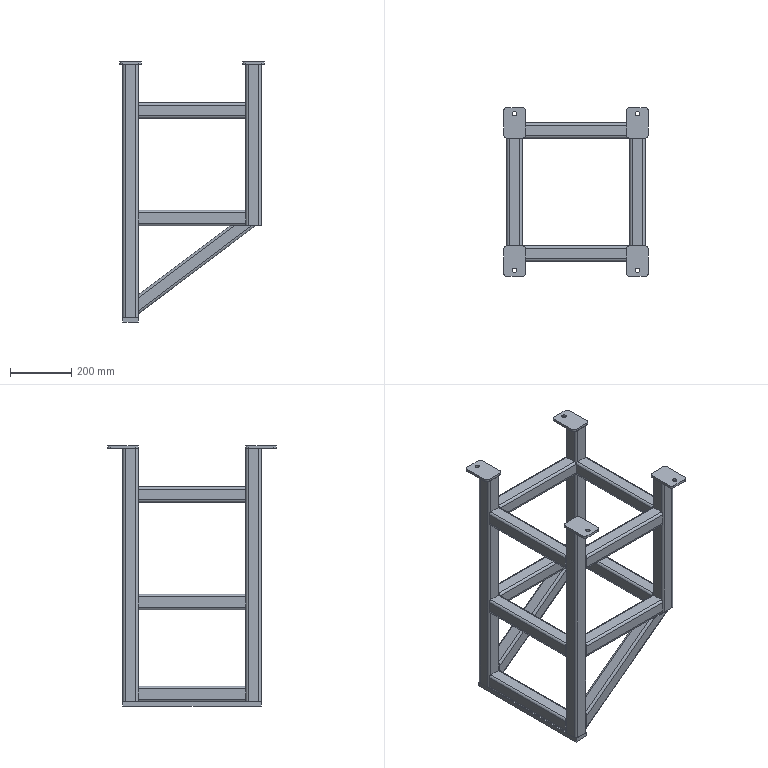Part | SolidWorks | features ReferencePattern 3, MirrorCompFeat 2 | 20 solids | 324 faces | box 470 x 550 x 847 mm | volume 5189358 mm3 | plane 180 | cylinder 144 | commonest cylinder face diameters 8 x60 16 x60 20 x16 14 x8